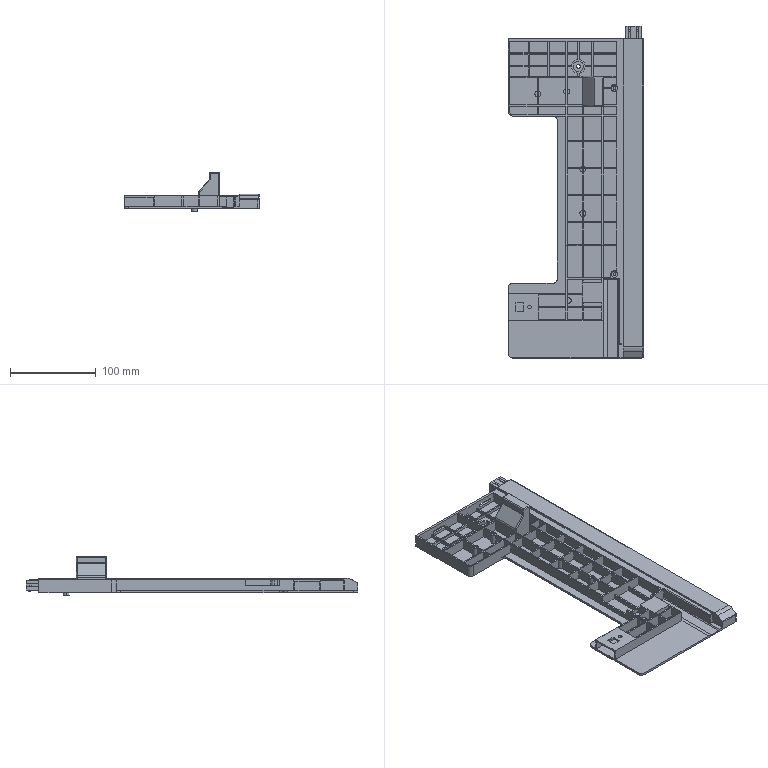Part | STEP file | ZXW722-L-25 | 1 solid | 544 faces | box 157.5 x 387 x 45.5 mm | volume 196671 mm3 | plane 433 | cylinder 97 | torus 7 | sphere 5 | spline 2 | commonest cylinder face diameters 2 x23 7 x19 4 x11 6 x10 40 x6 10 x5